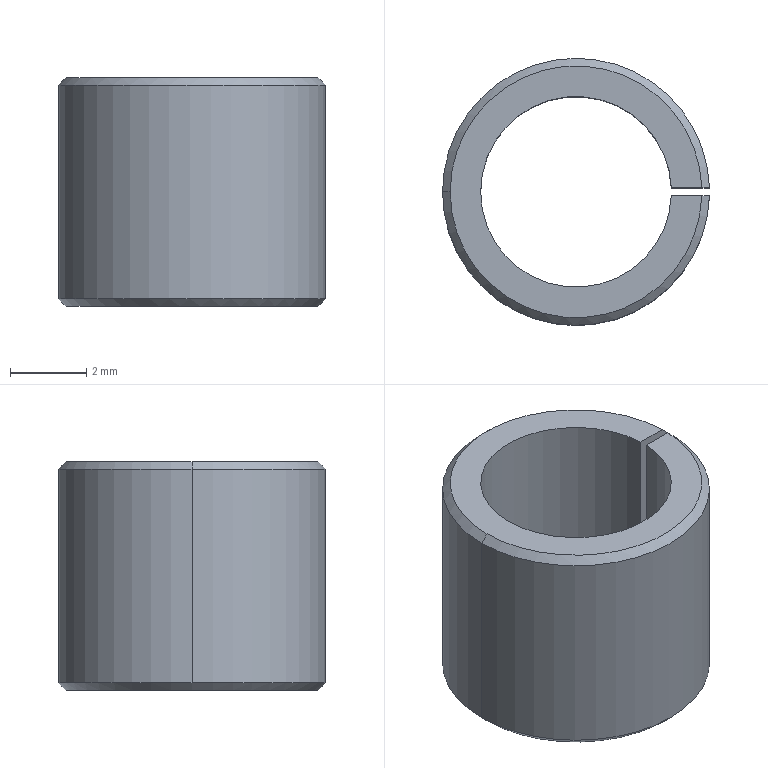Part | NX | features BREP 1 | 1 solid | 11 faces | box 6.999 x 7 x 6 mm | volume 111.042 mm3 | cylinder 4 | plane 4 | cone 3 | commonest cylinder face diameters 5 x2 7 x2
STEP:
#1=CARTESIAN_POINT('',(-3.3,0.,3.));
#2=VERTEX_POINT('',#1);
#3=CARTESIAN_POINT('',(3.298,-0.1,3.));
#4=VERTEX_POINT('',#3);
#5=CARTESIAN_POINT('',(0.,0.,3.));
#6=DIRECTION('',(0.,0.,1.));
#7=DIRECTION('',(1.,0.,0.));
#8=AXIS2_PLACEMENT_3D('',#5,#6,#7);
#9=CIRCLE('',#8,3.3);
#10=EDGE_CURVE('',#2,#4,#9,.T.);
#11=ORIENTED_EDGE('',*,*,#10,.F.);
#12=CARTESIAN_POINT('',(-3.5,0.,2.8));
#13=VERTEX_POINT('',#12);
#14=CARTESIAN_POINT('',(-3.3,0.,3.));
#15=DIRECTION('',(-0.7071,0.,-0.7071));
#16=VECTOR('',#15,1000.);
#17=LINE('',#14,#16);
#18=EDGE_CURVE('',#2,#13,#17,.T.);
#19=ORIENTED_EDGE('',*,*,#18,.T.);
#20=CARTESIAN_POINT('',(3.499,-0.1,2.8));
#21=VERTEX_POINT('',#20);
#22=CARTESIAN_POINT('',(0.,0.,2.8));
#23=DIRECTION('',(0.,0.,-1.));
#24=DIRECTION('',(1.,0.,0.));
#25=AXIS2_PLACEMENT_3D('',#22,#23,#24);
#26=CIRCLE('',#25,3.5);
#27=EDGE_CURVE('',#21,#13,#26,.T.);
#28=ORIENTED_EDGE('',*,*,#27,.F.);
#29=CARTESIAN_POINT('',(3.298,-0.1,3.));
#30=CARTESIAN_POINT('',(3.365,-0.1,2.933));
#31=CARTESIAN_POINT('',(3.432,-0.1,2.867));
#32=CARTESIAN_POINT('',(3.499,-0.1,2.8));
#33=B_SPLINE_CURVE_WITH_KNOTS('',3,(#29,#30,#31,#32),.UNSPECIFIED.,.F.,.F.,(4,4),(0.003879,0.004162),.UNSPECIFIED.);
#34=EDGE_CURVE('',#4,#21,#33,.T.);
#35=ORIENTED_EDGE('',*,*,#34,.F.);
#36=EDGE_LOOP('',(#11,#19,#28,#35));
#37=FACE_BOUND('',#36,.T.);
#38=CARTESIAN_POINT('',(0.,0.,3.));
#39=DIRECTION('',(0.,0.,-1.));
#40=DIRECTION('',(-1.,0.,0.));
#41=AXIS2_PLACEMENT_3D('',#38,#39,#40);
#42=CONICAL_SURFACE('',#41,3.3,0.7854);
#43=ADVANCED_FACE('',(#37),#42,.T.);
#44=CARTESIAN_POINT('',(2.498,0.1,3.));
#45=VERTEX_POINT('',#44);
#46=CARTESIAN_POINT('',(-2.5,0.,3.));
#47=VERTEX_POINT('',#46);
#48=CARTESIAN_POINT('',(0.,0.,3.));
#49=DIRECTION('',(0.,0.,1.));
#50=DIRECTION('',(1.,0.,0.));
#51=AXIS2_PLACEMENT_3D('',#48,#49,#50);
#52=CIRCLE('',#51,2.5);
#53=EDGE_CURVE('',#45,#47,#52,.T.);
#54=ORIENTED_EDGE('',*,*,#53,.T.);
#55=CARTESIAN_POINT('',(-2.5,0.,-3.));
#56=VERTEX_POINT('',#55);
#57=CARTESIAN_POINT('',(-2.5,0.,3.));
#58=DIRECTION('',(0.,0.,-1.));
#59=VECTOR('',#58,1000.);
#60=LINE('',#57,#59);
#61=EDGE_CURVE('',#47,#56,#60,.T.);
#62=ORIENTED_EDGE('',*,*,#61,.T.);
#63=CARTESIAN_POINT('',(2.498,0.1,-3.));
#64=VERTEX_POINT('',#63);
#65=CARTESIAN_POINT('',(0.,0.,-3.));
#66=DIRECTION('',(0.,0.,1.));
#67=DIRECTION('',(1.,0.,0.));
#68=AXIS2_PLACEMENT_3D('',#65,#66,#67);
#69=CIRCLE('',#68,2.5);
#70=EDGE_CURVE('',#64,#56,#69,.T.);
#71=ORIENTED_EDGE('',*,*,#70,.F.);
#72=CARTESIAN_POINT('',(2.498,0.1,3.));
#73=DIRECTION('',(0.,0.,-1.));
#74=VECTOR('',#73,1000.);
#75=LINE('',#72,#74);
#76=EDGE_CURVE('',#45,#64,#75,.T.);
#77=ORIENTED_EDGE('',*,*,#76,.F.);
#78=EDGE_LOOP('',(#54,#62,#71,#77));
#79=FACE_BOUND('',#78,.T.);
#80=CARTESIAN_POINT('',(0.,0.,3.));
#81=DIRECTION('',(0.,0.,-1.));
#82=DIRECTION('',(-1.,0.,0.));
#83=AXIS2_PLACEMENT_3D('',#80,#81,#82);
#84=CYLINDRICAL_SURFACE('',#83,2.5);
#85=ADVANCED_FACE('',(#79),#84,.F.);
#86=ORIENTED_EDGE('',*,*,#27,.T.);
#87=CARTESIAN_POINT('',(-3.5,0.,-2.8));
#88=VERTEX_POINT('',#87);
#89=CARTESIAN_POINT('',(-3.5,0.,3.));
#90=DIRECTION('',(0.,0.,-1.));
#91=VECTOR('',#90,1000.);
#92=LINE('',#89,#91);
#93=EDGE_CURVE('',#13,#88,#92,.T.);
#94=ORIENTED_EDGE('',*,*,#93,.T.);
#95=CARTESIAN_POINT('',(3.499,-0.1,-2.8));
#96=VERTEX_POINT('',#95);
#97=CARTESIAN_POINT('',(0.,0.,-2.8));
#98=DIRECTION('',(0.,0.,1.));
#99=DIRECTION('',(1.,0.,0.));
#100=AXIS2_PLACEMENT_3D('',#97,#98,#99);
#101=CIRCLE('',#100,3.5);
#102=EDGE_CURVE('',#88,#96,#101,.T.);
#103=ORIENTED_EDGE('',*,*,#102,.T.);
#104=CARTESIAN_POINT('',(3.499,-0.1,3.));
#105=DIRECTION('',(0.,0.,1.));
#106=VECTOR('',#105,1000.);
#107=LINE('',#104,#106);
#108=EDGE_CURVE('',#96,#21,#107,.T.);
#109=ORIENTED_EDGE('',*,*,#108,.T.);
#110=EDGE_LOOP('',(#86,#94,#103,#109));
#111=FACE_BOUND('',#110,.T.);
#112=CARTESIAN_POINT('',(0.,0.,3.));
#113=DIRECTION('',(0.,0.,-1.));
#114=DIRECTION('',(-1.,0.,0.));
#115=AXIS2_PLACEMENT_3D('',#112,#113,#114);
#116=CYLINDRICAL_SURFACE('',#115,3.5);
#117=ADVANCED_FACE('',(#111),#116,.T.);
#118=CARTESIAN_POINT('',(3.298,0.1,3.));
#119=VERTEX_POINT('',#118);
#120=CARTESIAN_POINT('',(0.,0.1,3.));
#121=DIRECTION('',(-1.,0.,0.));
#122=VECTOR('',#121,1000.);
#123=LINE('',#120,#122);
#124=EDGE_CURVE('',#119,#45,#123,.T.);
#125=ORIENTED_EDGE('',*,*,#124,.F.);
#126=CARTESIAN_POINT('',(0.,0.,3.));
#127=DIRECTION('',(0.,0.,1.));
#128=DIRECTION('',(1.,0.,0.));
#129=AXIS2_PLACEMENT_3D('',#126,#127,#128);
#130=CIRCLE('',#129,3.3);
#131=EDGE_CURVE('',#119,#2,#130,.T.);
#132=ORIENTED_EDGE('',*,*,#131,.T.);
#133=ORIENTED_EDGE('',*,*,#10,.T.);
#134=CARTESIAN_POINT('',(2.498,-0.1,3.));
#135=VERTEX_POINT('',#134);
#136=CARTESIAN_POINT('',(0.,-0.1,3.));
#137=DIRECTION('',(1.,0.,0.));
#138=VECTOR('',#137,1000.);
#139=LINE('',#136,#138);
#140=EDGE_CURVE('',#135,#4,#139,.T.);
#141=ORIENTED_EDGE('',*,*,#140,.F.);
#142=CARTESIAN_POINT('',(0.,0.,3.));
#143=DIRECTION('',(0.,0.,1.));
#144=DIRECTION('',(1.,0.,0.));
#145=AXIS2_PLACEMENT_3D('',#142,#143,#144);
#146=CIRCLE('',#145,2.5);
#147=EDGE_CURVE('',#47,#135,#146,.T.);
#148=ORIENTED_EDGE('',*,*,#147,.F.);
#149=ORIENTED_EDGE('',*,*,#53,.F.);
#150=EDGE_LOOP('',(#125,#132,#133,#141,#148,#149));
#151=FACE_BOUND('',#150,.T.);
#152=CARTESIAN_POINT('',(0.,0.,3.));
#153=DIRECTION('',(0.,0.,1.));
#154=DIRECTION('',(1.,0.,0.));
#155=AXIS2_PLACEMENT_3D('',#152,#153,#154);
#156=PLANE('',#155);
#157=ADVANCED_FACE('',(#151),#156,.T.);
#158=CARTESIAN_POINT('',(3.298,-0.1,-3.));
#159=VERTEX_POINT('',#158);
#160=CARTESIAN_POINT('',(3.298,0.1,-3.));
#161=VERTEX_POINT('',#160);
#162=CARTESIAN_POINT('',(0.,0.,-3.));
#163=DIRECTION('',(0.,0.,-1.));
#164=DIRECTION('',(1.,0.,0.));
#165=AXIS2_PLACEMENT_3D('',#162,#163,#164);
#166=CIRCLE('',#165,3.3);
#167=EDGE_CURVE('',#159,#161,#166,.T.);
#168=ORIENTED_EDGE('',*,*,#167,.T.);
#169=CARTESIAN_POINT('',(0.2567,0.1,-3.));
#170=DIRECTION('',(1.,0.,0.));
#171=VECTOR('',#170,1000.);
#172=LINE('',#169,#171);
#173=EDGE_CURVE('',#64,#161,#172,.T.);
#174=ORIENTED_EDGE('',*,*,#173,.F.);
#175=ORIENTED_EDGE('',*,*,#70,.T.);
#176=CARTESIAN_POINT('',(2.498,-0.1,-3.));
#177=VERTEX_POINT('',#176);
#178=CARTESIAN_POINT('',(0.,0.,-3.));
#179=DIRECTION('',(0.,0.,1.));
#180=DIRECTION('',(1.,0.,0.));
#181=AXIS2_PLACEMENT_3D('',#178,#179,#180);
#182=CIRCLE('',#181,2.5);
#183=EDGE_CURVE('',#56,#177,#182,.T.);
#184=ORIENTED_EDGE('',*,*,#183,.T.);
#185=CARTESIAN_POINT('',(0.2567,-0.1,-3.));
#186=DIRECTION('',(-1.,0.,0.));
#187=VECTOR('',#186,1000.);
#188=LINE('',#185,#187);
#189=EDGE_CURVE('',#159,#177,#188,.T.);
#190=ORIENTED_EDGE('',*,*,#189,.F.);
#191=EDGE_LOOP('',(#168,#174,#175,#184,#190));
#192=FACE_BOUND('',#191,.T.);
#193=CARTESIAN_POINT('',(0.,0.,-3.));
#194=DIRECTION('',(0.,0.,1.));
#195=DIRECTION('',(1.,0.,0.));
#196=AXIS2_PLACEMENT_3D('',#193,#194,#195);
#197=PLANE('',#196);
#198=ADVANCED_FACE('',(#192),#197,.F.);
#199=ORIENTED_EDGE('',*,*,#93,.F.);
#200=CARTESIAN_POINT('',(3.499,0.1,2.8));
#201=VERTEX_POINT('',#200);
#202=CARTESIAN_POINT('',(0.,0.,2.8));
#203=DIRECTION('',(0.,0.,-1.));
#204=DIRECTION('',(1.,0.,0.));
#205=AXIS2_PLACEMENT_3D('',#202,#203,#204);
#206=CIRCLE('',#205,3.5);
#207=EDGE_CURVE('',#13,#201,#206,.T.);
#208=ORIENTED_EDGE('',*,*,#207,.T.);
#209=CARTESIAN_POINT('',(3.499,0.1,-2.8));
#210=VERTEX_POINT('',#209);
#211=CARTESIAN_POINT('',(3.499,0.1,3.));
#212=DIRECTION('',(0.,0.,-1.));
#213=VECTOR('',#212,1000.);
#214=LINE('',#211,#213);
#215=EDGE_CURVE('',#201,#210,#214,.T.);
#216=ORIENTED_EDGE('',*,*,#215,.T.);
#217=CARTESIAN_POINT('',(0.,0.,-2.8));
#218=DIRECTION('',(0.,0.,1.));
#219=DIRECTION('',(1.,0.,0.));
#220=AXIS2_PLACEMENT_3D('',#217,#218,#219);
#221=CIRCLE('',#220,3.5);
#222=EDGE_CURVE('',#210,#88,#221,.T.);
#223=ORIENTED_EDGE('',*,*,#222,.T.);
#224=EDGE_LOOP('',(#199,#208,#216,#223));
#225=FACE_BOUND('',#224,.T.);
#226=CARTESIAN_POINT('',(0.,0.,3.));
#227=DIRECTION('',(0.,0.,-1.));
#228=DIRECTION('',(-1.,0.,0.));
#229=AXIS2_PLACEMENT_3D('',#226,#227,#228);
#230=CYLINDRICAL_SURFACE('',#229,3.5);
#231=ADVANCED_FACE('',(#225),#230,.T.);
#232=ORIENTED_EDGE('',*,*,#61,.F.);
#233=ORIENTED_EDGE('',*,*,#147,.T.);
#234=CARTESIAN_POINT('',(2.498,-0.1,3.));
#235=DIRECTION('',(0.,0.,1.));
#236=VECTOR('',#235,1000.);
#237=LINE('',#234,#236);
#238=EDGE_CURVE('',#177,#135,#237,.T.);
#239=ORIENTED_EDGE('',*,*,#238,.F.);
#240=ORIENTED_EDGE('',*,*,#183,.F.);
#241=EDGE_LOOP('',(#232,#233,#239,#240));
#242=FACE_BOUND('',#241,.T.);
#243=CARTESIAN_POINT('',(0.,0.,3.));
#244=DIRECTION('',(0.,0.,-1.));
#245=DIRECTION('',(-1.,0.,0.));
#246=AXIS2_PLACEMENT_3D('',#243,#244,#245);
#247=CYLINDRICAL_SURFACE('',#246,2.5);
#248=ADVANCED_FACE('',(#242),#247,.F.);
#249=CARTESIAN_POINT('',(3.298,0.1,-3.));
#250=CARTESIAN_POINT('',(3.365,0.1,-2.933));
#251=CARTESIAN_POINT('',(3.432,0.1,-2.867));
#252=CARTESIAN_POINT('',(3.499,0.1,-2.8));
#253=B_SPLINE_CURVE_WITH_KNOTS('',3,(#249,#250,#251,#252),.UNSPECIFIED.,.F.,.F.,(4,4),(0.003879,0.004162),.UNSPECIFIED.);
#254=EDGE_CURVE('',#161,#210,#253,.T.);
#255=ORIENTED_EDGE('',*,*,#254,.F.);
#256=ORIENTED_EDGE('',*,*,#167,.F.);
#257=CARTESIAN_POINT('',(3.499,-0.1,-2.8));
#258=CARTESIAN_POINT('',(3.432,-0.1,-2.867));
#259=CARTESIAN_POINT('',(3.365,-0.1,-2.933));
#260=CARTESIAN_POINT('',(3.298,-0.1,-3.));
#261=B_SPLINE_CURVE_WITH_KNOTS('',3,(#257,#258,#259,#260),.UNSPECIFIED.,.F.,.F.,(4,4),(0.003449,0.003732),.UNSPECIFIED.);
#262=EDGE_CURVE('',#96,#159,#261,.T.);
#263=ORIENTED_EDGE('',*,*,#262,.F.);
#264=ORIENTED_EDGE('',*,*,#102,.F.);
#265=ORIENTED_EDGE('',*,*,#222,.F.);
#266=EDGE_LOOP('',(#255,#256,#263,#264,#265));
#267=FACE_BOUND('',#266,.T.);
#268=CARTESIAN_POINT('',(0.,0.,-2.8));
#269=DIRECTION('',(0.,0.,1.));
#270=DIRECTION('',(1.,0.,0.));
#271=AXIS2_PLACEMENT_3D('',#268,#269,#270);
#272=CONICAL_SURFACE('',#271,3.5,0.7854);
#273=ADVANCED_FACE('',(#267),#272,.T.);
#274=ORIENTED_EDGE('',*,*,#18,.F.);
#275=ORIENTED_EDGE('',*,*,#131,.F.);
#276=CARTESIAN_POINT('',(3.499,0.1,2.8));
#277=CARTESIAN_POINT('',(3.432,0.1,2.867));
#278=CARTESIAN_POINT('',(3.365,0.1,2.933));
#279=CARTESIAN_POINT('',(3.298,0.1,3.));
#280=B_SPLINE_CURVE_WITH_KNOTS('',3,(#276,#277,#278,#279),.UNSPECIFIED.,.F.,.F.,(4,4),(0.003449,0.003732),.UNSPECIFIED.);
#281=EDGE_CURVE('',#201,#119,#280,.T.);
#282=ORIENTED_EDGE('',*,*,#281,.F.);
#283=ORIENTED_EDGE('',*,*,#207,.F.);
#284=EDGE_LOOP('',(#274,#275,#282,#283));
#285=FACE_BOUND('',#284,.T.);
#286=CARTESIAN_POINT('',(0.,0.,3.));
#287=DIRECTION('',(0.,0.,-1.));
#288=DIRECTION('',(-1.,0.,0.));
#289=AXIS2_PLACEMENT_3D('',#286,#287,#288);
#290=CONICAL_SURFACE('',#289,3.3,0.7854);
#291=ADVANCED_FACE('',(#285),#290,.T.);
#292=ORIENTED_EDGE('',*,*,#238,.T.);
#293=ORIENTED_EDGE('',*,*,#140,.T.);
#294=ORIENTED_EDGE('',*,*,#34,.T.);
#295=ORIENTED_EDGE('',*,*,#108,.F.);
#296=ORIENTED_EDGE('',*,*,#262,.T.);
#297=ORIENTED_EDGE('',*,*,#189,.T.);
#298=EDGE_LOOP('',(#292,#293,#294,#295,#296,#297));
#299=FACE_BOUND('',#298,.T.);
#300=CARTESIAN_POINT('',(0.2567,-0.1,7.));
#301=DIRECTION('',(0.,-1.,0.));
#302=DIRECTION('',(-1.,0.,0.));
#303=AXIS2_PLACEMENT_3D('',#300,#301,#302);
#304=PLANE('',#303);
#305=ADVANCED_FACE('',(#299),#304,.F.);
#306=ORIENTED_EDGE('',*,*,#76,.T.);
#307=ORIENTED_EDGE('',*,*,#173,.T.);
#308=ORIENTED_EDGE('',*,*,#254,.T.);
#309=ORIENTED_EDGE('',*,*,#215,.F.);
#310=ORIENTED_EDGE('',*,*,#281,.T.);
#311=ORIENTED_EDGE('',*,*,#124,.T.);
#312=EDGE_LOOP('',(#306,#307,#308,#309,#310,#311));
#313=FACE_BOUND('',#312,.T.);
#314=CARTESIAN_POINT('',(0.2567,0.1,7.));
#315=DIRECTION('',(0.,1.,0.));
#316=DIRECTION('',(1.,0.,0.));
#317=AXIS2_PLACEMENT_3D('',#314,#315,#316);
#318=PLANE('',#317);
#319=ADVANCED_FACE('',(#313),#318,.F.);
#320=CLOSED_SHELL('',(#43,#85,#117,#157,#198,#231,#248,#273,#291,#305,#319));
#321=MANIFOLD_SOLID_BREP('',#320);
#322=(LENGTH_UNIT()NAMED_UNIT(*)SI_UNIT(.MILLI.,.METRE.));
#323=UNCERTAINTY_MEASURE_WITH_UNIT(LENGTH_MEASURE(0.00001),#322,'','');
#324=(NAMED_UNIT(*)PLANE_ANGLE_UNIT()SI_UNIT($,.RADIAN.));
#325=(NAMED_UNIT(*)SI_UNIT($,.STERADIAN.)SOLID_ANGLE_UNIT());
#326=(GEOMETRIC_REPRESENTATION_CONTEXT(3)GLOBAL_UNCERTAINTY_ASSIGNED_CONTEXT((#323))GLOBAL_UNIT_ASSIGNED_CONTEXT((#322,#324,#325))REPRESENTATION_CONTEXT('',''));
#327=ADVANCED_BREP_SHAPE_REPRESENTATION('',(#321),#326);